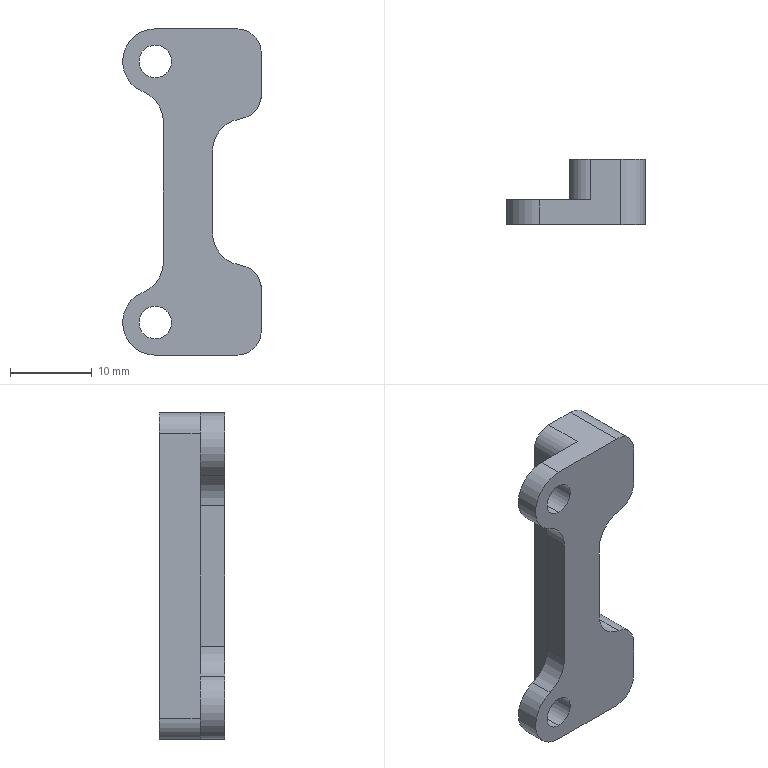NC program | Mastercam | posted with a generic post | part box 17 x 8 x 40 mm
Lines 1 to 24 of 8055:
%
:0001()
(MATERIAL - ALUMINUM MM - 2024)
(T24|100 FEM |H24)
(T8|8 FEM |H8|XY STOCK TO LEAVE - .1|Z STOCK TO LEAVE - 0.)
(T7|4 CHM |H7)
N100 G21
N102 G0 G17 G40 G80 G90 G94 G98
N104 G0 G28 G91 Z0.
N106 G0 G28 X0. Y0.
(100 FEM |TOOL - 24|DIA. OFF. - 24|LEN. - 24|TOOL DIA. - 100.)
N108 T24 M6
N110 G0 G54 G90 X-105. Y0. C0. B0. S4000 M3
N112 G43 H24 Z50.
N114 Z2.
N116 G1 Z0. F600.
N118 X105. F1000.
N120 G0 Z50.
N122 M5
N124 G0 G28 G91 Z0.
N126 G28
N128 M01
N130 G0 G17 G40 G80 G90 G94 G98
N132 G0 G28 G91 Z0.